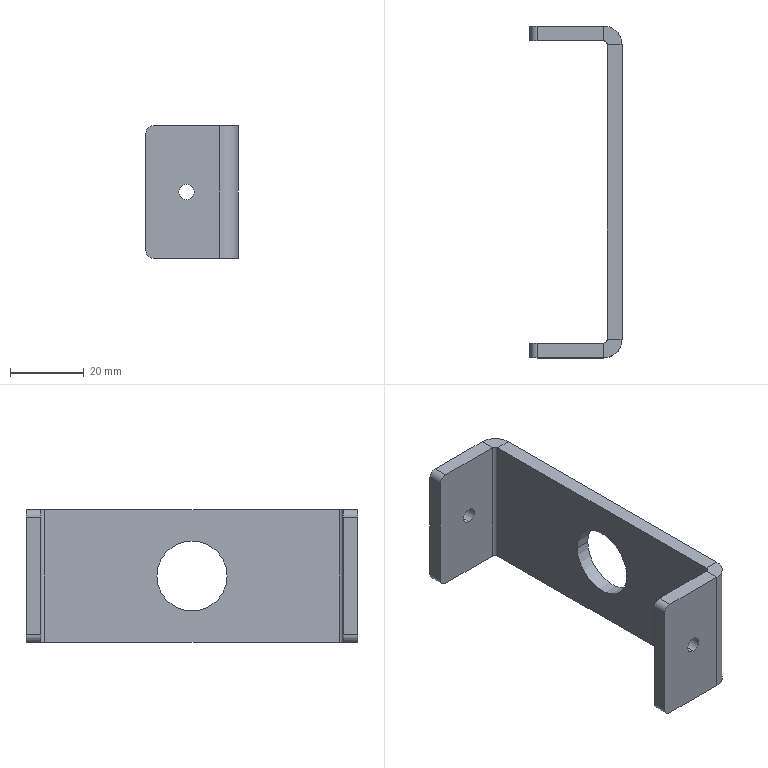Part | STEP file | Cang dai | 1 solid | 32 faces | box 25 x 90 x 36 mm | volume 17378 mm3 | plane 18 | cylinder 14 | commonest cylinder face diameters 4 x4 4.2 x4 2 x2 10 x2 19 x2
STEP:
#1=CARTESIAN_POINT('',(-4.,9.5,0.));
#2=VERTEX_POINT('',#1);
#3=CARTESIAN_POINT('',(-4.,-9.5,0.));
#4=VERTEX_POINT('',#3);
#5=CARTESIAN_POINT('',(-4.,0.,0.));
#6=DIRECTION('',(-1.,0.,0.));
#7=DIRECTION('',(0.,0.,1.));
#8=AXIS2_PLACEMENT_3D('',#5,#6,#7);
#9=CIRCLE('',#8,9.5);
#10=EDGE_CURVE('',#2,#4,#9,.T.);
#11=ORIENTED_EDGE('',*,*,#10,.T.);
#12=CARTESIAN_POINT('',(0.,-9.5,0.));
#13=VERTEX_POINT('',#12);
#14=CARTESIAN_POINT('',(-25.,-9.5,0.));
#15=DIRECTION('',(1.,0.,0.));
#16=VECTOR('',#15,1000.);
#17=LINE('',#14,#16);
#18=EDGE_CURVE('',#4,#13,#17,.T.);
#19=ORIENTED_EDGE('',*,*,#18,.T.);
#20=CARTESIAN_POINT('',(0.,9.5,0.));
#21=VERTEX_POINT('',#20);
#22=CARTESIAN_POINT('',(0.,0.,0.));
#23=DIRECTION('',(1.,0.,0.));
#24=DIRECTION('',(0.,1.,0.));
#25=AXIS2_PLACEMENT_3D('',#22,#23,#24);
#26=CIRCLE('',#25,9.5);
#27=EDGE_CURVE('',#13,#21,#26,.T.);
#28=ORIENTED_EDGE('',*,*,#27,.T.);
#29=CARTESIAN_POINT('',(-25.,9.5,0.));
#30=DIRECTION('',(1.,0.,0.));
#31=VECTOR('',#30,1000.);
#32=LINE('',#29,#31);
#33=EDGE_CURVE('',#2,#21,#32,.T.);
#34=ORIENTED_EDGE('',*,*,#33,.F.);
#35=EDGE_LOOP('',(#11,#19,#28,#34));
#36=FACE_OUTER_BOUND('',#35,.T.);
#37=CARTESIAN_POINT('',(-25.,0.,0.));
#38=DIRECTION('',(1.,0.,0.));
#39=DIRECTION('',(0.,1.,0.));
#40=AXIS2_PLACEMENT_3D('',#37,#38,#39);
#41=CYLINDRICAL_SURFACE('',#40,9.5);
#42=ADVANCED_FACE('',(#36),#41,.F.);
#43=CARTESIAN_POINT('',(-14.,-41.,-2.1));
#44=VERTEX_POINT('',#43);
#45=CARTESIAN_POINT('',(-14.,-41.,2.1));
#46=VERTEX_POINT('',#45);
#47=CARTESIAN_POINT('',(-14.,-41.,0.));
#48=DIRECTION('',(0.,1.,0.));
#49=DIRECTION('',(0.,0.,1.));
#50=AXIS2_PLACEMENT_3D('',#47,#48,#49);
#51=CIRCLE('',#50,2.1);
#52=EDGE_CURVE('',#44,#46,#51,.T.);
#53=ORIENTED_EDGE('',*,*,#52,.T.);
#54=CARTESIAN_POINT('',(-14.,-45.,2.1));
#55=VERTEX_POINT('',#54);
#56=CARTESIAN_POINT('',(-14.,-45.,2.1));
#57=DIRECTION('',(0.,-1.,0.));
#58=VECTOR('',#57,1000.);
#59=LINE('',#56,#58);
#60=EDGE_CURVE('',#46,#55,#59,.T.);
#61=ORIENTED_EDGE('',*,*,#60,.T.);
#62=CARTESIAN_POINT('',(-14.,-45.,-2.1));
#63=VERTEX_POINT('',#62);
#64=CARTESIAN_POINT('',(-14.,-45.,0.));
#65=DIRECTION('',(0.,-1.,0.));
#66=DIRECTION('',(0.,0.,-1.));
#67=AXIS2_PLACEMENT_3D('',#64,#65,#66);
#68=CIRCLE('',#67,2.1);
#69=EDGE_CURVE('',#55,#63,#68,.T.);
#70=ORIENTED_EDGE('',*,*,#69,.T.);
#71=CARTESIAN_POINT('',(-14.,-45.,-2.1));
#72=DIRECTION('',(0.,-1.,0.));
#73=VECTOR('',#72,1000.);
#74=LINE('',#71,#73);
#75=EDGE_CURVE('',#44,#63,#74,.T.);
#76=ORIENTED_EDGE('',*,*,#75,.F.);
#77=EDGE_LOOP('',(#53,#61,#70,#76));
#78=FACE_OUTER_BOUND('',#77,.T.);
#79=CARTESIAN_POINT('',(-14.,-45.,0.));
#80=DIRECTION('',(0.,-1.,0.));
#81=DIRECTION('',(0.,0.,-1.));
#82=AXIS2_PLACEMENT_3D('',#79,#80,#81);
#83=CYLINDRICAL_SURFACE('',#82,2.1);
#84=ADVANCED_FACE('',(#78),#83,.F.);
#85=CARTESIAN_POINT('',(-14.,41.,2.1));
#86=VERTEX_POINT('',#85);
#87=CARTESIAN_POINT('',(-14.,41.,-2.1));
#88=VERTEX_POINT('',#87);
#89=CARTESIAN_POINT('',(-14.,41.,0.));
#90=DIRECTION('',(0.,-1.,0.));
#91=DIRECTION('',(0.,0.,-1.));
#92=AXIS2_PLACEMENT_3D('',#89,#90,#91);
#93=CIRCLE('',#92,2.1);
#94=EDGE_CURVE('',#86,#88,#93,.T.);
#95=ORIENTED_EDGE('',*,*,#94,.T.);
#96=CARTESIAN_POINT('',(-14.,45.,-2.1));
#97=VERTEX_POINT('',#96);
#98=CARTESIAN_POINT('',(-14.,45.,-2.1));
#99=DIRECTION('',(0.,1.,0.));
#100=VECTOR('',#99,1000.);
#101=LINE('',#98,#100);
#102=EDGE_CURVE('',#88,#97,#101,.T.);
#103=ORIENTED_EDGE('',*,*,#102,.T.);
#104=CARTESIAN_POINT('',(-14.,45.,2.1));
#105=VERTEX_POINT('',#104);
#106=CARTESIAN_POINT('',(-14.,45.,0.));
#107=DIRECTION('',(0.,1.,0.));
#108=DIRECTION('',(0.,0.,1.));
#109=AXIS2_PLACEMENT_3D('',#106,#107,#108);
#110=CIRCLE('',#109,2.1);
#111=EDGE_CURVE('',#97,#105,#110,.T.);
#112=ORIENTED_EDGE('',*,*,#111,.T.);
#113=CARTESIAN_POINT('',(-14.,45.,2.1));
#114=DIRECTION('',(0.,1.,0.));
#115=VECTOR('',#114,1000.);
#116=LINE('',#113,#115);
#117=EDGE_CURVE('',#86,#105,#116,.T.);
#118=ORIENTED_EDGE('',*,*,#117,.F.);
#119=EDGE_LOOP('',(#95,#103,#112,#118));
#120=FACE_OUTER_BOUND('',#119,.T.);
#121=CARTESIAN_POINT('',(-14.,45.,0.));
#122=DIRECTION('',(0.,1.,0.));
#123=DIRECTION('',(0.,0.,1.));
#124=AXIS2_PLACEMENT_3D('',#121,#122,#123);
#125=CYLINDRICAL_SURFACE('',#124,2.1);
#126=ADVANCED_FACE('',(#120),#125,.F.);
#127=CARTESIAN_POINT('',(-25.,-45.,16.));
#128=VERTEX_POINT('',#127);
#129=CARTESIAN_POINT('',(-25.,-45.,-16.));
#130=VERTEX_POINT('',#129);
#131=CARTESIAN_POINT('',(-25.,-45.,18.));
#132=DIRECTION('',(0.,0.,-1.));
#133=VECTOR('',#132,1000.);
#134=LINE('',#131,#133);
#135=EDGE_CURVE('',#128,#130,#134,.T.);
#136=ORIENTED_EDGE('',*,*,#135,.T.);
#137=CARTESIAN_POINT('',(-23.,-45.,-18.));
#138=VERTEX_POINT('',#137);
#139=CARTESIAN_POINT('',(-23.,-45.,-16.));
#140=DIRECTION('',(0.,-1.,0.));
#141=DIRECTION('',(0.,0.,1.));
#142=AXIS2_PLACEMENT_3D('',#139,#140,#141);
#143=CIRCLE('',#142,2.);
#144=EDGE_CURVE('',#130,#138,#143,.T.);
#145=ORIENTED_EDGE('',*,*,#144,.T.);
#146=CARTESIAN_POINT('',(-5.,-45.,-18.));
#147=VERTEX_POINT('',#146);
#148=CARTESIAN_POINT('',(0.,-45.,-18.));
#149=DIRECTION('',(1.,0.,0.));
#150=VECTOR('',#149,1000.);
#151=LINE('',#148,#150);
#152=EDGE_CURVE('',#138,#147,#151,.T.);
#153=ORIENTED_EDGE('',*,*,#152,.T.);
#154=CARTESIAN_POINT('',(-5.,-45.,18.));
#155=VERTEX_POINT('',#154);
#156=CARTESIAN_POINT('',(-5.,-45.,18.));
#157=DIRECTION('',(0.,0.,-1.));
#158=VECTOR('',#157,1000.);
#159=LINE('',#156,#158);
#160=EDGE_CURVE('',#155,#147,#159,.T.);
#161=ORIENTED_EDGE('',*,*,#160,.F.);
#162=CARTESIAN_POINT('',(-23.,-45.,18.));
#163=VERTEX_POINT('',#162);
#164=CARTESIAN_POINT('',(0.,-45.,18.));
#165=DIRECTION('',(1.,0.,0.));
#166=VECTOR('',#165,1000.);
#167=LINE('',#164,#166);
#168=EDGE_CURVE('',#163,#155,#167,.T.);
#169=ORIENTED_EDGE('',*,*,#168,.F.);
#170=CARTESIAN_POINT('',(-23.,-45.,16.));
#171=DIRECTION('',(0.,-1.,0.));
#172=DIRECTION('',(0.,0.,1.));
#173=AXIS2_PLACEMENT_3D('',#170,#171,#172);
#174=CIRCLE('',#173,2.);
#175=EDGE_CURVE('',#163,#128,#174,.T.);
#176=ORIENTED_EDGE('',*,*,#175,.T.);
#177=EDGE_LOOP('',(#136,#145,#153,#161,#169,#176));
#178=FACE_OUTER_BOUND('',#177,.T.);
#179=CARTESIAN_POINT('',(-14.,-45.,0.));
#180=DIRECTION('',(0.,-1.,0.));
#181=DIRECTION('',(0.,0.,-1.));
#182=AXIS2_PLACEMENT_3D('',#179,#180,#181);
#183=CIRCLE('',#182,2.1);
#184=EDGE_CURVE('',#63,#55,#183,.T.);
#185=ORIENTED_EDGE('',*,*,#184,.F.);
#186=ORIENTED_EDGE('',*,*,#69,.F.);
#187=EDGE_LOOP('',(#185,#186));
#188=FACE_BOUND('',#187,.T.);
#189=CARTESIAN_POINT('',(0.,-45.,18.));
#190=DIRECTION('',(0.,1.,0.));
#191=DIRECTION('',(0.,0.,1.));
#192=AXIS2_PLACEMENT_3D('',#189,#190,#191);
#193=PLANE('',#192);
#194=ADVANCED_FACE('',(#178,#188),#193,.F.);
#195=CARTESIAN_POINT('',(-5.,45.,-18.));
#196=VERTEX_POINT('',#195);
#197=CARTESIAN_POINT('',(-23.,45.,-18.));
#198=VERTEX_POINT('',#197);
#199=CARTESIAN_POINT('',(0.,45.,-18.));
#200=DIRECTION('',(-1.,0.,0.));
#201=VECTOR('',#200,1000.);
#202=LINE('',#199,#201);
#203=EDGE_CURVE('',#196,#198,#202,.T.);
#204=ORIENTED_EDGE('',*,*,#203,.T.);
#205=CARTESIAN_POINT('',(-25.,45.,-16.));
#206=VERTEX_POINT('',#205);
#207=CARTESIAN_POINT('',(-23.,45.,-16.));
#208=DIRECTION('',(0.,1.,0.));
#209=DIRECTION('',(0.,0.,-1.));
#210=AXIS2_PLACEMENT_3D('',#207,#208,#209);
#211=CIRCLE('',#210,2.);
#212=EDGE_CURVE('',#198,#206,#211,.T.);
#213=ORIENTED_EDGE('',*,*,#212,.T.);
#214=CARTESIAN_POINT('',(-25.,45.,16.));
#215=VERTEX_POINT('',#214);
#216=CARTESIAN_POINT('',(-25.,45.,18.));
#217=DIRECTION('',(0.,0.,-1.));
#218=VECTOR('',#217,1000.);
#219=LINE('',#216,#218);
#220=EDGE_CURVE('',#215,#206,#219,.T.);
#221=ORIENTED_EDGE('',*,*,#220,.F.);
#222=CARTESIAN_POINT('',(-23.,45.,18.));
#223=VERTEX_POINT('',#222);
#224=CARTESIAN_POINT('',(-23.,45.,16.));
#225=DIRECTION('',(0.,1.,0.));
#226=DIRECTION('',(0.,0.,-1.));
#227=AXIS2_PLACEMENT_3D('',#224,#225,#226);
#228=CIRCLE('',#227,2.);
#229=EDGE_CURVE('',#215,#223,#228,.T.);
#230=ORIENTED_EDGE('',*,*,#229,.T.);
#231=CARTESIAN_POINT('',(-5.,45.,18.));
#232=VERTEX_POINT('',#231);
#233=CARTESIAN_POINT('',(0.,45.,18.));
#234=DIRECTION('',(-1.,0.,0.));
#235=VECTOR('',#234,1000.);
#236=LINE('',#233,#235);
#237=EDGE_CURVE('',#232,#223,#236,.T.);
#238=ORIENTED_EDGE('',*,*,#237,.F.);
#239=CARTESIAN_POINT('',(-5.,45.,18.));
#240=DIRECTION('',(0.,0.,-1.));
#241=VECTOR('',#240,1000.);
#242=LINE('',#239,#241);
#243=EDGE_CURVE('',#232,#196,#242,.T.);
#244=ORIENTED_EDGE('',*,*,#243,.T.);
#245=EDGE_LOOP('',(#204,#213,#221,#230,#238,#244));
#246=FACE_OUTER_BOUND('',#245,.T.);
#247=CARTESIAN_POINT('',(-14.,45.,0.));
#248=DIRECTION('',(0.,1.,0.));
#249=DIRECTION('',(0.,0.,1.));
#250=AXIS2_PLACEMENT_3D('',#247,#248,#249);
#251=CIRCLE('',#250,2.1);
#252=EDGE_CURVE('',#105,#97,#251,.T.);
#253=ORIENTED_EDGE('',*,*,#252,.F.);
#254=ORIENTED_EDGE('',*,*,#111,.F.);
#255=EDGE_LOOP('',(#253,#254));
#256=FACE_BOUND('',#255,.T.);
#257=CARTESIAN_POINT('',(0.,45.,18.));
#258=DIRECTION('',(0.,-1.,0.));
#259=DIRECTION('',(0.,0.,-1.));
#260=AXIS2_PLACEMENT_3D('',#257,#258,#259);
#261=PLANE('',#260);
#262=ADVANCED_FACE('',(#246,#256),#261,.F.);
#263=CARTESIAN_POINT('',(-5.,-41.,18.));
#264=VERTEX_POINT('',#263);
#265=CARTESIAN_POINT('',(-5.,-45.,18.));
#266=DIRECTION('',(0.,1.,0.));
#267=VECTOR('',#266,1000.);
#268=LINE('',#265,#267);
#269=EDGE_CURVE('',#155,#264,#268,.T.);
#270=ORIENTED_EDGE('',*,*,#269,.F.);
#271=CARTESIAN_POINT('',(0.,-40.,18.));
#272=VERTEX_POINT('',#271);
#273=CARTESIAN_POINT('',(-5.,-40.,18.));
#274=DIRECTION('',(0.,0.,1.));
#275=DIRECTION('',(-1.,0.,0.));
#276=AXIS2_PLACEMENT_3D('',#273,#274,#275);
#277=CIRCLE('',#276,5.);
#278=EDGE_CURVE('',#155,#272,#277,.T.);
#279=ORIENTED_EDGE('',*,*,#278,.T.);
#280=CARTESIAN_POINT('',(-4.,-40.,18.));
#281=VERTEX_POINT('',#280);
#282=CARTESIAN_POINT('',(-4.,-40.,18.));
#283=DIRECTION('',(1.,0.,0.));
#284=VECTOR('',#283,1000.);
#285=LINE('',#282,#284);
#286=EDGE_CURVE('',#281,#272,#285,.T.);
#287=ORIENTED_EDGE('',*,*,#286,.F.);
#288=CARTESIAN_POINT('',(-5.,-40.,18.));
#289=DIRECTION('',(0.,0.,1.));
#290=DIRECTION('',(1.,0.,0.));
#291=AXIS2_PLACEMENT_3D('',#288,#289,#290);
#292=CIRCLE('',#291,1.);
#293=EDGE_CURVE('',#264,#281,#292,.T.);
#294=ORIENTED_EDGE('',*,*,#293,.F.);
#295=EDGE_LOOP('',(#270,#279,#287,#294));
#296=FACE_OUTER_BOUND('',#295,.T.);
#297=CARTESIAN_POINT('',(-5.,-45.,18.));
#298=DIRECTION('',(0.,0.,1.));
#299=DIRECTION('',(1.,0.,0.));
#300=AXIS2_PLACEMENT_3D('',#297,#298,#299);
#301=PLANE('',#300);
#302=ADVANCED_FACE('',(#296),#301,.T.);
#303=CARTESIAN_POINT('',(-23.,-41.,18.));
#304=VERTEX_POINT('',#303);
#305=CARTESIAN_POINT('',(0.,-41.,18.));
#306=DIRECTION('',(1.,0.,0.));
#307=VECTOR('',#306,1000.);
#308=LINE('',#305,#307);
#309=EDGE_CURVE('',#304,#264,#308,.T.);
#310=ORIENTED_EDGE('',*,*,#309,.F.);
#311=CARTESIAN_POINT('',(-23.,-40.,18.));
#312=DIRECTION('',(0.,-1.,0.));
#313=VECTOR('',#312,1000.);
#314=LINE('',#311,#313);
#315=EDGE_CURVE('',#304,#163,#314,.T.);
#316=ORIENTED_EDGE('',*,*,#315,.T.);
#317=ORIENTED_EDGE('',*,*,#168,.T.);
#318=ORIENTED_EDGE('',*,*,#269,.T.);
#319=EDGE_LOOP('',(#310,#316,#317,#318));
#320=FACE_OUTER_BOUND('',#319,.T.);
#321=CARTESIAN_POINT('',(-4.,-40.,18.));
#322=DIRECTION('',(0.,0.,1.));
#323=DIRECTION('',(1.,0.,0.));
#324=AXIS2_PLACEMENT_3D('',#321,#322,#323);
#325=PLANE('',#324);
#326=ADVANCED_FACE('',(#320),#325,.T.);
#327=CARTESIAN_POINT('',(0.,-40.,-18.));
#328=VERTEX_POINT('',#327);
#329=CARTESIAN_POINT('',(-4.,-40.,-18.));
#330=VERTEX_POINT('',#329);
#331=CARTESIAN_POINT('',(0.,-40.,-18.));
#332=DIRECTION('',(-1.,0.,0.));
#333=VECTOR('',#332,1000.);
#334=LINE('',#331,#333);
#335=EDGE_CURVE('',#328,#330,#334,.T.);
#336=ORIENTED_EDGE('',*,*,#335,.F.);
#337=CARTESIAN_POINT('',(-5.,-40.,-18.));
#338=DIRECTION('',(0.,0.,1.));
#339=DIRECTION('',(-1.,0.,0.));
#340=AXIS2_PLACEMENT_3D('',#337,#338,#339);
#341=CIRCLE('',#340,5.);
#342=EDGE_CURVE('',#147,#328,#341,.T.);
#343=ORIENTED_EDGE('',*,*,#342,.F.);
#344=CARTESIAN_POINT('',(-5.,-41.,-18.));
#345=VERTEX_POINT('',#344);
#346=CARTESIAN_POINT('',(-5.,-41.,-18.));
#347=DIRECTION('',(0.,-1.,0.));
#348=VECTOR('',#347,1000.);
#349=LINE('',#346,#348);
#350=EDGE_CURVE('',#345,#147,#349,.T.);
#351=ORIENTED_EDGE('',*,*,#350,.F.);
#352=CARTESIAN_POINT('',(-5.,-40.,-18.));
#353=DIRECTION('',(0.,0.,1.));
#354=DIRECTION('',(1.,0.,0.));
#355=AXIS2_PLACEMENT_3D('',#352,#353,#354);
#356=CIRCLE('',#355,1.);
#357=EDGE_CURVE('',#345,#330,#356,.T.);
#358=ORIENTED_EDGE('',*,*,#357,.T.);
#359=EDGE_LOOP('',(#336,#343,#351,#358));
#360=FACE_OUTER_BOUND('',#359,.T.);
#361=CARTESIAN_POINT('',(0.,-40.,-18.));
#362=DIRECTION('',(0.,0.,-1.));
#363=DIRECTION('',(-1.,0.,0.));
#364=AXIS2_PLACEMENT_3D('',#361,#362,#363);
#365=PLANE('',#364);
#366=ADVANCED_FACE('',(#360),#365,.T.);
#367=CARTESIAN_POINT('',(0.,40.,-18.));
#368=VERTEX_POINT('',#367);
#369=CARTESIAN_POINT('',(0.,45.,-18.));
#370=DIRECTION('',(0.,1.,0.));
#371=VECTOR('',#370,1000.);
#372=LINE('',#369,#371);
#373=EDGE_CURVE('',#328,#368,#372,.T.);
#374=ORIENTED_EDGE('',*,*,#373,.F.);
#375=ORIENTED_EDGE('',*,*,#335,.T.);
#376=CARTESIAN_POINT('',(-4.,40.,-18.));
#377=VERTEX_POINT('',#376);
#378=CARTESIAN_POINT('',(-4.,45.,-18.));
#379=DIRECTION('',(0.,1.,0.));
#380=VECTOR('',#379,1000.);
#381=LINE('',#378,#380);
#382=EDGE_CURVE('',#330,#377,#381,.T.);
#383=ORIENTED_EDGE('',*,*,#382,.T.);
#384=CARTESIAN_POINT('',(-4.,40.,-18.));
#385=DIRECTION('',(1.,0.,0.));
#386=VECTOR('',#385,1000.);
#387=LINE('',#384,#386);
#388=EDGE_CURVE('',#377,#368,#387,.T.);
#389=ORIENTED_EDGE('',*,*,#388,.T.);
#390=EDGE_LOOP('',(#374,#375,#383,#389));
#391=FACE_OUTER_BOUND('',#390,.T.);
#392=CARTESIAN_POINT('',(-5.,-41.,-18.));
#393=DIRECTION('',(0.,0.,-1.));
#394=DIRECTION('',(-1.,0.,0.));
#395=AXIS2_PLACEMENT_3D('',#392,#393,#394);
#396=PLANE('',#395);
#397=ADVANCED_FACE('',(#391),#396,.T.);
#398=CARTESIAN_POINT('',(0.,40.,18.));
#399=VERTEX_POINT('',#398);
#400=CARTESIAN_POINT('',(-4.,40.,18.));
#401=VERTEX_POINT('',#400);
#402=CARTESIAN_POINT('',(0.,40.,18.));
#403=DIRECTION('',(-1.,0.,0.));
#404=VECTOR('',#403,1000.);
#405=LINE('',#402,#404);
#406=EDGE_CURVE('',#399,#401,#405,.T.);
#407=ORIENTED_EDGE('',*,*,#406,.F.);
#408=CARTESIAN_POINT('',(-5.,40.,18.));
#409=DIRECTION('',(0.,0.,1.));
#410=DIRECTION('',(-1.,0.,0.));
#411=AXIS2_PLACEMENT_3D('',#408,#409,#410);
#412=CIRCLE('',#411,5.);
#413=EDGE_CURVE('',#399,#232,#412,.T.);
#414=ORIENTED_EDGE('',*,*,#413,.T.);
#415=CARTESIAN_POINT('',(-5.,41.,18.));
#416=VERTEX_POINT('',#415);
#417=CARTESIAN_POINT('',(-5.,41.,18.));
#418=DIRECTION('',(0.,1.,0.));
#419=VECTOR('',#418,1000.);
#420=LINE('',#417,#419);
#421=EDGE_CURVE('',#416,#232,#420,.T.);
#422=ORIENTED_EDGE('',*,*,#421,.F.);
#423=CARTESIAN_POINT('',(-5.,40.,18.));
#424=DIRECTION('',(0.,0.,1.));
#425=DIRECTION('',(1.,0.,0.));
#426=AXIS2_PLACEMENT_3D('',#423,#424,#425);
#427=CIRCLE('',#426,1.);
#428=EDGE_CURVE('',#401,#416,#427,.T.);
#429=ORIENTED_EDGE('',*,*,#428,.F.);
#430=EDGE_LOOP('',(#407,#414,#422,#429));
#431=FACE_OUTER_BOUND('',#430,.T.);
#432=CARTESIAN_POINT('',(0.,40.,18.));
#433=DIRECTION('',(0.,0.,1.));
#434=DIRECTION('',(1.,0.,0.));
#435=AXIS2_PLACEMENT_3D('',#432,#433,#434);
#436=PLANE('',#435);
#437=ADVANCED_FACE('',(#431),#436,.T.);
#438=CARTESIAN_POINT('',(0.,45.,18.));
#439=DIRECTION('',(0.,1.,0.));
#440=VECTOR('',#439,1000.);
#441=LINE('',#438,#440);
#442=EDGE_CURVE('',#272,#399,#441,.T.);
#443=ORIENTED_EDGE('',*,*,#442,.T.);
#444=ORIENTED_EDGE('',*,*,#406,.T.);
#445=CARTESIAN_POINT('',(-4.,45.,18.));
#446=DIRECTION('',(0.,1.,0.));
#447=VECTOR('',#446,1000.);
#448=LINE('',#445,#447);
#449=EDGE_CURVE('',#281,#401,#448,.T.);
#450=ORIENTED_EDGE('',*,*,#449,.F.);
#451=ORIENTED_EDGE('',*,*,#286,.T.);
#452=EDGE_LOOP('',(#443,#444,#450,#451));
#453=FACE_OUTER_BOUND('',#452,.T.);
#454=CARTESIAN_POINT('',(-5.,41.,18.));
#455=DIRECTION('',(0.,0.,1.));
#456=DIRECTION('',(1.,0.,0.));
#457=AXIS2_PLACEMENT_3D('',#454,#455,#456);
#458=PLANE('',#457);
#459=ADVANCED_FACE('',(#453),#458,.T.);
#460=CARTESIAN_POINT('',(-5.,41.,-18.));
#461=VERTEX_POINT('',#460);
#462=CARTESIAN_POINT('',(-5.,45.,-18.));
#463=DIRECTION('',(0.,-1.,0.));
#464=VECTOR('',#463,1000.);
#465=LINE('',#462,#464);
#466=EDGE_CURVE('',#196,#461,#465,.T.);
#467=ORIENTED_EDGE('',*,*,#466,.F.);
#468=CARTESIAN_POINT('',(-5.,40.,-18.));
#469=DIRECTION('',(0.,0.,1.));
#470=DIRECTION('',(-1.,0.,0.));
#471=AXIS2_PLACEMENT_3D('',#468,#469,#470);
#472=CIRCLE('',#471,5.);
#473=EDGE_CURVE('',#368,#196,#472,.T.);
#474=ORIENTED_EDGE('',*,*,#473,.F.);
#475=ORIENTED_EDGE('',*,*,#388,.F.);
#476=CARTESIAN_POINT('',(-5.,40.,-18.));
#477=DIRECTION('',(0.,0.,1.));
#478=DIRECTION('',(1.,0.,0.));
#479=AXIS2_PLACEMENT_3D('',#476,#477,#478);
#480=CIRCLE('',#479,1.);
#481=EDGE_CURVE('',#377,#461,#480,.T.);
#482=ORIENTED_EDGE('',*,*,#481,.T.);
#483=EDGE_LOOP('',(#467,#474,#475,#482));
#484=FACE_OUTER_BOUND('',#483,.T.);
#485=CARTESIAN_POINT('',(-5.,45.,-18.));
#486=DIRECTION('',(0.,0.,-1.));
#487=DIRECTION('',(-1.,0.,0.));
#488=AXIS2_PLACEMENT_3D('',#485,#486,#487);
#489=PLANE('',#488);
#490=ADVANCED_FACE('',(#484),#489,.T.);
#491=CARTESIAN_POINT('',(-23.,41.,-18.));
#492=VERTEX_POINT('',#491);
#493=CARTESIAN_POINT('',(0.,41.,-18.));
#494=DIRECTION('',(-1.,0.,0.));
#495=VECTOR('',#494,1000.);
#496=LINE('',#493,#495);
#497=EDGE_CURVE('',#461,#492,#496,.T.);
#498=ORIENTED_EDGE('',*,*,#497,.T.);
#499=CARTESIAN_POINT('',(-23.,40.,-18.));
#500=DIRECTION('',(0.,1.,0.));
#501=VECTOR('',#500,1000.);
#502=LINE('',#499,#501);
#503=EDGE_CURVE('',#492,#198,#502,.T.);
#504=ORIENTED_EDGE('',*,*,#503,.T.);
#505=ORIENTED_EDGE('',*,*,#203,.F.);
#506=ORIENTED_EDGE('',*,*,#466,.T.);
#507=EDGE_LOOP('',(#498,#504,#505,#506));
#508=FACE_OUTER_BOUND('',#507,.T.);
#509=CARTESIAN_POINT('',(-4.,40.,-18.));
#510=DIRECTION('',(0.,0.,-1.));
#511=DIRECTION('',(-1.,0.,0.));
#512=AXIS2_PLACEMENT_3D('',#509,#510,#511);
#513=PLANE('',#512);
#514=ADVANCED_FACE('',(#508),#513,.T.);
#515=ORIENTED_EDGE('',*,*,#220,.T.);
#516=CARTESIAN_POINT('',(-25.,41.,-16.));
#517=VERTEX_POINT('',#516);
#518=CARTESIAN_POINT('',(-25.,41.,-16.));
#519=DIRECTION('',(0.,-1.,0.));
#520=VECTOR('',#519,1000.);
#521=LINE('',#518,#520);
#522=EDGE_CURVE('',#206,#517,#521,.T.);
#523=ORIENTED_EDGE('',*,*,#522,.T.);
#524=CARTESIAN_POINT('',(-25.,41.,16.));
#525=VERTEX_POINT('',#524);
#526=CARTESIAN_POINT('',(-25.,41.,18.));
#527=DIRECTION('',(0.,0.,-1.));
#528=VECTOR('',#527,1000.);
#529=LINE('',#526,#528);
#530=EDGE_CURVE('',#525,#517,#529,.T.);
#531=ORIENTED_EDGE('',*,*,#530,.F.);
#532=CARTESIAN_POINT('',(-25.,41.,16.));
#533=DIRECTION('',(0.,1.,0.));
#534=VECTOR('',#533,1000.);
#535=LINE('',#532,#534);
#536=EDGE_CURVE('',#525,#215,#535,.T.);
#537=ORIENTED_EDGE('',*,*,#536,.T.);
#538=EDGE_LOOP('',(#515,#523,#531,#537));
#539=FACE_OUTER_BOUND('',#538,.T.);
#540=CARTESIAN_POINT('',(-25.,41.,18.));
#541=DIRECTION('',(-1.,0.,0.));
#542=DIRECTION('',(0.,0.,1.));
#543=AXIS2_PLACEMENT_3D('',#540,#541,#542);
#544=PLANE('',#543);
#545=ADVANCED_FACE('',(#539),#544,.T.);
#546=ORIENTED_EDGE('',*,*,#94,.F.);
#547=CARTESIAN_POINT('',(-14.,41.,0.));
#548=DIRECTION('',(0.,-1.,0.));
#549=DIRECTION('',(0.,0.,-1.));
#550=AXIS2_PLACEMENT_3D('',#547,#548,#549);
#551=CIRCLE('',#550,2.1);
#552=EDGE_CURVE('',#88,#86,#551,.T.);
#553=ORIENTED_EDGE('',*,*,#552,.F.);
#554=EDGE_LOOP('',(#546,#553));
#555=FACE_BOUND('',#554,.T.);
#556=ORIENTED_EDGE('',*,*,#530,.T.);
#557=CARTESIAN_POINT('',(-23.,41.,-16.));
#558=DIRECTION('',(0.,-1.,0.));
#559=DIRECTION('',(0.,0.,-1.));
#560=AXIS2_PLACEMENT_3D('',#557,#558,#559);
#561=CIRCLE('',#560,2.);
#562=EDGE_CURVE('',#517,#492,#561,.T.);
#563=ORIENTED_EDGE('',*,*,#562,.T.);
#564=ORIENTED_EDGE('',*,*,#497,.F.);
#565=CARTESIAN_POINT('',(-5.,41.,18.));
#566=DIRECTION('',(0.,0.,-1.));
#567=VECTOR('',#566,1000.);
#568=LINE('',#565,#567);
#569=EDGE_CURVE('',#416,#461,#568,.T.);
#570=ORIENTED_EDGE('',*,*,#569,.F.);
#571=CARTESIAN_POINT('',(-23.,41.,18.));
#572=VERTEX_POINT('',#571);
#573=CARTESIAN_POINT('',(0.,41.,18.));
#574=DIRECTION('',(-1.,0.,0.));
#575=VECTOR('',#574,1000.);
#576=LINE('',#573,#575);
#577=EDGE_CURVE('',#416,#572,#576,.T.);
#578=ORIENTED_EDGE('',*,*,#577,.T.);
#579=CARTESIAN_POINT('',(-23.,41.,16.));
#580=DIRECTION('',(0.,-1.,0.));
#581=DIRECTION('',(0.,0.,-1.));
#582=AXIS2_PLACEMENT_3D('',#579,#580,#581);
#583=CIRCLE('',#582,2.);
#584=EDGE_CURVE('',#572,#525,#583,.T.);
#585=ORIENTED_EDGE('',*,*,#584,.T.);
#586=EDGE_LOOP('',(#556,#563,#564,#570,#578,#585));
#587=FACE_OUTER_BOUND('',#586,.T.);
#588=CARTESIAN_POINT('',(0.,41.,18.));
#589=DIRECTION('',(0.,-1.,0.));
#590=DIRECTION('',(0.,0.,-1.));
#591=AXIS2_PLACEMENT_3D('',#588,#589,#590);
#592=PLANE('',#591);
#593=ADVANCED_FACE('',(#555,#587),#592,.T.);
#594=ORIENTED_EDGE('',*,*,#481,.F.);
#595=CARTESIAN_POINT('',(-4.,40.,18.));
#596=DIRECTION('',(0.,0.,-1.));
#597=VECTOR('',#596,1000.);
#598=LINE('',#595,#597);
#599=EDGE_CURVE('',#401,#377,#598,.T.);
#600=ORIENTED_EDGE('',*,*,#599,.F.);
#601=ORIENTED_EDGE('',*,*,#428,.T.);
#602=ORIENTED_EDGE('',*,*,#569,.T.);
#603=EDGE_LOOP('',(#594,#600,#601,#602));
#604=FACE_OUTER_BOUND('',#603,.T.);
#605=CARTESIAN_POINT('',(-5.,40.,18.));
#606=DIRECTION('',(0.,0.,-1.));
#607=DIRECTION('',(-1.,0.,0.));
#608=AXIS2_PLACEMENT_3D('',#605,#606,#607);
#609=CYLINDRICAL_SURFACE('',#608,1.);
#610=ADVANCED_FACE('',(#604),#609,.F.);
#611=ORIENTED_EDGE('',*,*,#10,.F.);
#612=CARTESIAN_POINT('',(-4.,0.,0.));
#613=DIRECTION('',(-1.,0.,0.));
#614=DIRECTION('',(0.,0.,1.));
#615=AXIS2_PLACEMENT_3D('',#612,#613,#614);
#616=CIRCLE('',#615,9.5);
#617=EDGE_CURVE('',#4,#2,#616,.T.);
#618=ORIENTED_EDGE('',*,*,#617,.F.);
#619=EDGE_LOOP('',(#611,#618));
#620=FACE_BOUND('',#619,.T.);
#621=ORIENTED_EDGE('',*,*,#382,.F.);
#622=CARTESIAN_POINT('',(-4.,-40.,18.));
#623=DIRECTION('',(0.,0.,-1.));
#624=VECTOR('',#623,1000.);
#625=LINE('',#622,#624);
#626=EDGE_CURVE('',#281,#330,#625,.T.);
#627=ORIENTED_EDGE('',*,*,#626,.F.);
#628=ORIENTED_EDGE('',*,*,#449,.T.);
#629=ORIENTED_EDGE('',*,*,#599,.T.);
#630=EDGE_LOOP('',(#621,#627,#628,#629));
#631=FACE_OUTER_BOUND('',#630,.T.);
#632=CARTESIAN_POINT('',(-4.,45.,18.));
#633=DIRECTION('',(-1.,0.,0.));
#634=DIRECTION('',(0.,0.,1.));
#635=AXIS2_PLACEMENT_3D('',#632,#633,#634);
#636=PLANE('',#635);
#637=ADVANCED_FACE('',(#620,#631),#636,.T.);
#638=ORIENTED_EDGE('',*,*,#357,.F.);
#639=CARTESIAN_POINT('',(-5.,-41.,18.));
#640=DIRECTION('',(0.,0.,-1.));
#641=VECTOR('',#640,1000.);
#642=LINE('',#639,#641);
#643=EDGE_CURVE('',#264,#345,#642,.T.);
#644=ORIENTED_EDGE('',*,*,#643,.F.);
#645=ORIENTED_EDGE('',*,*,#293,.T.);
#646=ORIENTED_EDGE('',*,*,#626,.T.);
#647=EDGE_LOOP('',(#638,#644,#645,#646));
#648=FACE_OUTER_BOUND('',#647,.T.);
#649=CARTESIAN_POINT('',(-5.,-40.,18.));
#650=DIRECTION('',(0.,0.,-1.));
#651=DIRECTION('',(-1.,0.,0.));
#652=AXIS2_PLACEMENT_3D('',#649,#650,#651);
#653=CYLINDRICAL_SURFACE('',#652,1.);
#654=ADVANCED_FACE('',(#648),#653,.F.);
#655=ORIENTED_EDGE('',*,*,#52,.F.);
#656=CARTESIAN_POINT('',(-14.,-41.,0.));
#657=DIRECTION('',(0.,1.,0.));
#658=DIRECTION('',(0.,0.,1.));
#659=AXIS2_PLACEMENT_3D('',#656,#657,#658);
#660=CIRCLE('',#659,2.1);
#661=EDGE_CURVE('',#46,#44,#660,.T.);
#662=ORIENTED_EDGE('',*,*,#661,.F.);
#663=EDGE_LOOP('',(#655,#662));
#664=FACE_BOUND('',#663,.T.);
#665=CARTESIAN_POINT('',(-23.,-41.,-18.));
#666=VERTEX_POINT('',#665);
#667=CARTESIAN_POINT('',(0.,-41.,-18.));
#668=DIRECTION('',(1.,0.,0.));
#669=VECTOR('',#668,1000.);
#670=LINE('',#667,#669);
#671=EDGE_CURVE('',#666,#345,#670,.T.);
#672=ORIENTED_EDGE('',*,*,#671,.F.);
#673=CARTESIAN_POINT('',(-25.,-41.,-16.));
#674=VERTEX_POINT('',#673);
#675=CARTESIAN_POINT('',(-23.,-41.,-16.));
#676=DIRECTION('',(0.,1.,0.));
#677=DIRECTION('',(0.,0.,1.));
#678=AXIS2_PLACEMENT_3D('',#675,#676,#677);
#679=CIRCLE('',#678,2.);
#680=EDGE_CURVE('',#666,#674,#679,.T.);
#681=ORIENTED_EDGE('',*,*,#680,.T.);
#682=CARTESIAN_POINT('',(-25.,-41.,16.));
#683=VERTEX_POINT('',#682);
#684=CARTESIAN_POINT('',(-25.,-41.,18.));
#685=DIRECTION('',(0.,0.,-1.));
#686=VECTOR('',#685,1000.);
#687=LINE('',#684,#686);
#688=EDGE_CURVE('',#683,#674,#687,.T.);
#689=ORIENTED_EDGE('',*,*,#688,.F.);
#690=CARTESIAN_POINT('',(-23.,-41.,16.));
#691=DIRECTION('',(0.,1.,0.));
#692=DIRECTION('',(0.,0.,1.));
#693=AXIS2_PLACEMENT_3D('',#690,#691,#692);
#694=CIRCLE('',#693,2.);
#695=EDGE_CURVE('',#683,#304,#694,.T.);
#696=ORIENTED_EDGE('',*,*,#695,.T.);
#697=ORIENTED_EDGE('',*,*,#309,.T.);
#698=ORIENTED_EDGE('',*,*,#643,.T.);
#699=EDGE_LOOP('',(#672,#681,#689,#696,#697,#698));
#700=FACE_OUTER_BOUND('',#699,.T.);
#701=CARTESIAN_POINT('',(0.,-41.,18.));
#702=DIRECTION('',(0.,1.,0.));
#703=DIRECTION('',(0.,0.,1.));
#704=AXIS2_PLACEMENT_3D('',#701,#702,#703);
#705=PLANE('',#704);
#706=ADVANCED_FACE('',(#664,#700),#705,.T.);
#707=ORIENTED_EDGE('',*,*,#688,.T.);
#708=CARTESIAN_POINT('',(-25.,-45.,-16.));
#709=DIRECTION('',(0.,-1.,0.));
#710=VECTOR('',#709,1000.);
#711=LINE('',#708,#710);
#712=EDGE_CURVE('',#674,#130,#711,.T.);
#713=ORIENTED_EDGE('',*,*,#712,.T.);
#714=ORIENTED_EDGE('',*,*,#135,.F.);
#715=CARTESIAN_POINT('',(-25.,-45.,16.));
#716=DIRECTION('',(0.,1.,0.));
#717=VECTOR('',#716,1000.);
#718=LINE('',#715,#717);
#719=EDGE_CURVE('',#128,#683,#718,.T.);
#720=ORIENTED_EDGE('',*,*,#719,.T.);
#721=EDGE_LOOP('',(#707,#713,#714,#720));
#722=FACE_OUTER_BOUND('',#721,.T.);
#723=CARTESIAN_POINT('',(-25.,-45.,18.));
#724=DIRECTION('',(-1.,0.,0.));
#725=DIRECTION('',(0.,0.,1.));
#726=AXIS2_PLACEMENT_3D('',#723,#724,#725);
#727=PLANE('',#726);
#728=ADVANCED_FACE('',(#722),#727,.T.);
#729=ORIENTED_EDGE('',*,*,#342,.T.);
#730=CARTESIAN_POINT('',(0.,-40.,18.));
#731=DIRECTION('',(0.,0.,-1.));
#732=VECTOR('',#731,1000.);
#733=LINE('',#730,#732);
#734=EDGE_CURVE('',#272,#328,#733,.T.);
#735=ORIENTED_EDGE('',*,*,#734,.F.);
#736=ORIENTED_EDGE('',*,*,#278,.F.);
#737=ORIENTED_EDGE('',*,*,#160,.T.);
#738=EDGE_LOOP('',(#729,#735,#736,#737));
#739=FACE_OUTER_BOUND('',#738,.T.);
#740=CARTESIAN_POINT('',(-5.,-40.,18.));
#741=DIRECTION('',(0.,0.,-1.));
#742=DIRECTION('',(-1.,0.,0.));
#743=AXIS2_PLACEMENT_3D('',#740,#741,#742);
#744=CYLINDRICAL_SURFACE('',#743,5.);
#745=ADVANCED_FACE('',(#739),#744,.T.);
#746=CARTESIAN_POINT('',(0.,0.,0.));
#747=DIRECTION('',(1.,0.,0.));
#748=DIRECTION('',(0.,1.,0.));
#749=AXIS2_PLACEMENT_3D('',#746,#747,#748);
#750=CIRCLE('',#749,9.5);
#751=EDGE_CURVE('',#21,#13,#750,.T.);
#752=ORIENTED_EDGE('',*,*,#751,.F.);
#753=ORIENTED_EDGE('',*,*,#27,.F.);
#754=EDGE_LOOP('',(#752,#753));
#755=FACE_BOUND('',#754,.T.);
#756=ORIENTED_EDGE('',*,*,#373,.T.);
#757=CARTESIAN_POINT('',(0.,40.,18.));
#758=DIRECTION('',(0.,0.,-1.));
#759=VECTOR('',#758,1000.);
#760=LINE('',#757,#759);
#761=EDGE_CURVE('',#399,#368,#760,.T.);
#762=ORIENTED_EDGE('',*,*,#761,.F.);
#763=ORIENTED_EDGE('',*,*,#442,.F.);
#764=ORIENTED_EDGE('',*,*,#734,.T.);
#765=EDGE_LOOP('',(#756,#762,#763,#764));
#766=FACE_OUTER_BOUND('',#765,.T.);
#767=CARTESIAN_POINT('',(0.,45.,18.));
#768=DIRECTION('',(-1.,0.,0.));
#769=DIRECTION('',(0.,0.,1.));
#770=AXIS2_PLACEMENT_3D('',#767,#768,#769);
#771=PLANE('',#770);
#772=ADVANCED_FACE('',(#755,#766),#771,.F.);
#773=ORIENTED_EDGE('',*,*,#473,.T.);
#774=ORIENTED_EDGE('',*,*,#243,.F.);
#775=ORIENTED_EDGE('',*,*,#413,.F.);
#776=ORIENTED_EDGE('',*,*,#761,.T.);
#777=EDGE_LOOP('',(#773,#774,#775,#776));
#778=FACE_OUTER_BOUND('',#777,.T.);
#779=CARTESIAN_POINT('',(-5.,40.,18.));
#780=DIRECTION('',(0.,0.,-1.));
#781=DIRECTION('',(-1.,0.,0.));
#782=AXIS2_PLACEMENT_3D('',#779,#780,#781);
#783=CYLINDRICAL_SURFACE('',#782,5.);
#784=ADVANCED_FACE('',(#778),#783,.T.);
#785=ORIENTED_EDGE('',*,*,#237,.T.);
#786=CARTESIAN_POINT('',(-23.,40.,18.));
#787=DIRECTION('',(0.,-1.,0.));
#788=VECTOR('',#787,1000.);
#789=LINE('',#786,#788);
#790=EDGE_CURVE('',#223,#572,#789,.T.);
#791=ORIENTED_EDGE('',*,*,#790,.T.);
#792=ORIENTED_EDGE('',*,*,#577,.F.);
#793=ORIENTED_EDGE('',*,*,#421,.T.);
#794=EDGE_LOOP('',(#785,#791,#792,#793));
#795=FACE_OUTER_BOUND('',#794,.T.);
#796=CARTESIAN_POINT('',(-5.,40.,18.));
#797=DIRECTION('',(0.,0.,1.));
#798=DIRECTION('',(1.,0.,0.));
#799=AXIS2_PLACEMENT_3D('',#796,#797,#798);
#800=PLANE('',#799);
#801=ADVANCED_FACE('',(#795),#800,.T.);
#802=ORIENTED_EDGE('',*,*,#152,.F.);
#803=CARTESIAN_POINT('',(-23.,-41.,-18.));
#804=DIRECTION('',(0.,1.,0.));
#805=VECTOR('',#804,1000.);
#806=LINE('',#803,#805);
#807=EDGE_CURVE('',#138,#666,#806,.T.);
#808=ORIENTED_EDGE('',*,*,#807,.T.);
#809=ORIENTED_EDGE('',*,*,#671,.T.);
#810=ORIENTED_EDGE('',*,*,#350,.T.);
#811=EDGE_LOOP('',(#802,#808,#809,#810));
#812=FACE_OUTER_BOUND('',#811,.T.);
#813=CARTESIAN_POINT('',(-5.,40.,-18.));
#814=DIRECTION('',(0.,0.,1.));
#815=DIRECTION('',(1.,0.,0.));
#816=AXIS2_PLACEMENT_3D('',#813,#814,#815);
#817=PLANE('',#816);
#818=ADVANCED_FACE('',(#812),#817,.F.);
#819=ORIENTED_EDGE('',*,*,#144,.F.);
#820=ORIENTED_EDGE('',*,*,#712,.F.);
#821=ORIENTED_EDGE('',*,*,#680,.F.);
#822=ORIENTED_EDGE('',*,*,#807,.F.);
#823=EDGE_LOOP('',(#819,#820,#821,#822));
#824=FACE_OUTER_BOUND('',#823,.T.);
#825=CARTESIAN_POINT('',(-23.,40.,-16.));
#826=DIRECTION('',(0.,-1.,0.));
#827=DIRECTION('',(0.,0.,-1.));
#828=AXIS2_PLACEMENT_3D('',#825,#826,#827);
#829=CYLINDRICAL_SURFACE('',#828,2.);
#830=ADVANCED_FACE('',(#824),#829,.T.);
#831=ORIENTED_EDGE('',*,*,#175,.F.);
#832=ORIENTED_EDGE('',*,*,#315,.F.);
#833=ORIENTED_EDGE('',*,*,#695,.F.);
#834=ORIENTED_EDGE('',*,*,#719,.F.);
#835=EDGE_LOOP('',(#831,#832,#833,#834));
#836=FACE_OUTER_BOUND('',#835,.T.);
#837=CARTESIAN_POINT('',(-23.,-45.,16.));
#838=DIRECTION('',(0.,1.,0.));
#839=DIRECTION('',(0.,0.,1.));
#840=AXIS2_PLACEMENT_3D('',#837,#838,#839);
#841=CYLINDRICAL_SURFACE('',#840,2.);
#842=ADVANCED_FACE('',(#836),#841,.T.);
#843=ORIENTED_EDGE('',*,*,#562,.F.);
#844=ORIENTED_EDGE('',*,*,#522,.F.);
#845=ORIENTED_EDGE('',*,*,#212,.F.);
#846=ORIENTED_EDGE('',*,*,#503,.F.);
#847=EDGE_LOOP('',(#843,#844,#845,#846));
#848=FACE_OUTER_BOUND('',#847,.T.);
#849=CARTESIAN_POINT('',(-23.,40.,-16.));
#850=DIRECTION('',(0.,1.,0.));
#851=DIRECTION('',(0.,0.,1.));
#852=AXIS2_PLACEMENT_3D('',#849,#850,#851);
#853=CYLINDRICAL_SURFACE('',#852,2.);
#854=ADVANCED_FACE('',(#848),#853,.T.);
#855=ORIENTED_EDGE('',*,*,#584,.F.);
#856=ORIENTED_EDGE('',*,*,#790,.F.);
#857=ORIENTED_EDGE('',*,*,#229,.F.);
#858=ORIENTED_EDGE('',*,*,#536,.F.);
#859=EDGE_LOOP('',(#855,#856,#857,#858));
#860=FACE_OUTER_BOUND('',#859,.T.);
#861=CARTESIAN_POINT('',(-23.,41.,16.));
#862=DIRECTION('',(0.,1.,0.));
#863=DIRECTION('',(0.,0.,1.));
#864=AXIS2_PLACEMENT_3D('',#861,#862,#863);
#865=CYLINDRICAL_SURFACE('',#864,2.);
#866=ADVANCED_FACE('',(#860),#865,.T.);
#867=ORIENTED_EDGE('',*,*,#102,.F.);
#868=ORIENTED_EDGE('',*,*,#552,.T.);
#869=ORIENTED_EDGE('',*,*,#117,.T.);
#870=ORIENTED_EDGE('',*,*,#252,.T.);
#871=EDGE_LOOP('',(#867,#868,#869,#870));
#872=FACE_OUTER_BOUND('',#871,.T.);
#873=CARTESIAN_POINT('',(-14.,45.,0.));
#874=DIRECTION('',(0.,1.,0.));
#875=DIRECTION('',(0.,0.,1.));
#876=AXIS2_PLACEMENT_3D('',#873,#874,#875);
#877=CYLINDRICAL_SURFACE('',#876,2.1);
#878=ADVANCED_FACE('',(#872),#877,.F.);
#879=ORIENTED_EDGE('',*,*,#60,.F.);
#880=ORIENTED_EDGE('',*,*,#661,.T.);
#881=ORIENTED_EDGE('',*,*,#75,.T.);
#882=ORIENTED_EDGE('',*,*,#184,.T.);
#883=EDGE_LOOP('',(#879,#880,#881,#882));
#884=FACE_OUTER_BOUND('',#883,.T.);
#885=CARTESIAN_POINT('',(-14.,-45.,0.));
#886=DIRECTION('',(0.,-1.,0.));
#887=DIRECTION('',(0.,0.,-1.));
#888=AXIS2_PLACEMENT_3D('',#885,#886,#887);
#889=CYLINDRICAL_SURFACE('',#888,2.1);
#890=ADVANCED_FACE('',(#884),#889,.F.);
#891=ORIENTED_EDGE('',*,*,#18,.F.);
#892=ORIENTED_EDGE('',*,*,#617,.T.);
#893=ORIENTED_EDGE('',*,*,#33,.T.);
#894=ORIENTED_EDGE('',*,*,#751,.T.);
#895=EDGE_LOOP('',(#891,#892,#893,#894));
#896=FACE_OUTER_BOUND('',#895,.T.);
#897=CARTESIAN_POINT('',(-25.,0.,0.));
#898=DIRECTION('',(1.,0.,0.));
#899=DIRECTION('',(0.,1.,0.));
#900=AXIS2_PLACEMENT_3D('',#897,#898,#899);
#901=CYLINDRICAL_SURFACE('',#900,9.5);
#902=ADVANCED_FACE('',(#896),#901,.F.);
#903=CLOSED_SHELL('',(#42,#84,#126,#194,#262,#302,#326,#366,#397,#437,#459,#490,#514,#545,#593,#610,#637,#654,#706,#728,#745,#772,#784,#801,#818,#830,#842,#854,#866,#878,#890,#902));
#904=MANIFOLD_SOLID_BREP('',#903);
#905=CARTESIAN_POINT('',(0.,0.,0.));
#906=DIRECTION('',(0.,0.,1.));
#907=DIRECTION('',(1.,0.,0.));
#908=AXIS2_PLACEMENT_3D('',#905,#906,#907);
#909=(LENGTH_UNIT()NAMED_UNIT(*)SI_UNIT(.MILLI.,.METRE.));
#910=UNCERTAINTY_MEASURE_WITH_UNIT(LENGTH_MEASURE(0.00001),#909,'','');
#911=(NAMED_UNIT(*)PLANE_ANGLE_UNIT()SI_UNIT($,.RADIAN.));
#912=(NAMED_UNIT(*)SI_UNIT($,.STERADIAN.)SOLID_ANGLE_UNIT());
#913=(GEOMETRIC_REPRESENTATION_CONTEXT(3)GLOBAL_UNCERTAINTY_ASSIGNED_CONTEXT((#910))GLOBAL_UNIT_ASSIGNED_CONTEXT((#909,#911,#912))REPRESENTATION_CONTEXT('',''));
#914=ADVANCED_BREP_SHAPE_REPRESENTATION('',(#904,#908),#913);